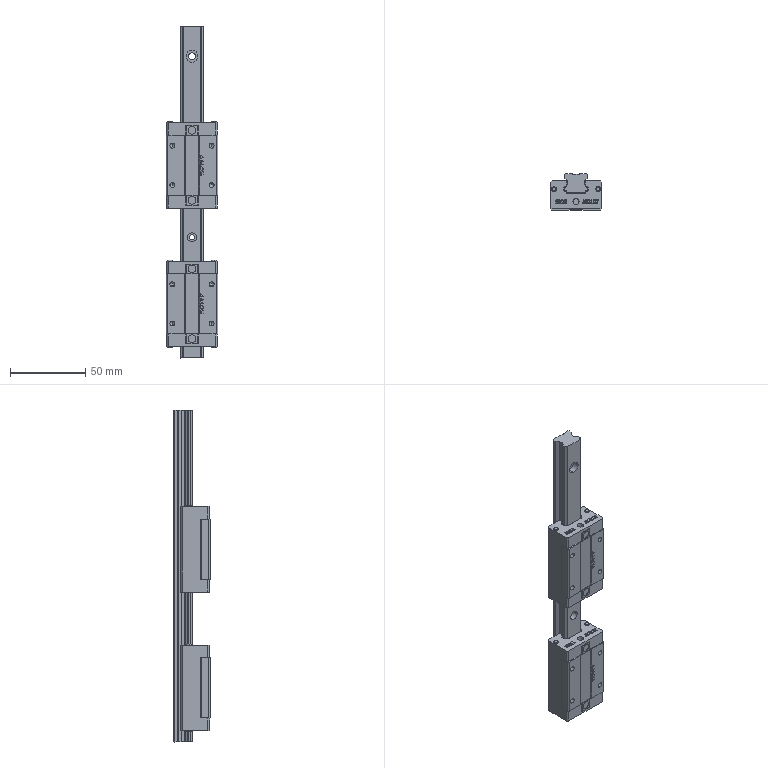Part | SolidWorks | 3 solids | 1021 faces | box 34 x 24 x 220 mm | volume 96136 mm3 | plane 687 | cylinder 164 | spline 138 | torus 16 | cone 16 | commonest cylinder face diameters 1.6 x32 2.1 x24 0.6 x19 0.46 x16 3.3 x16 3 x15